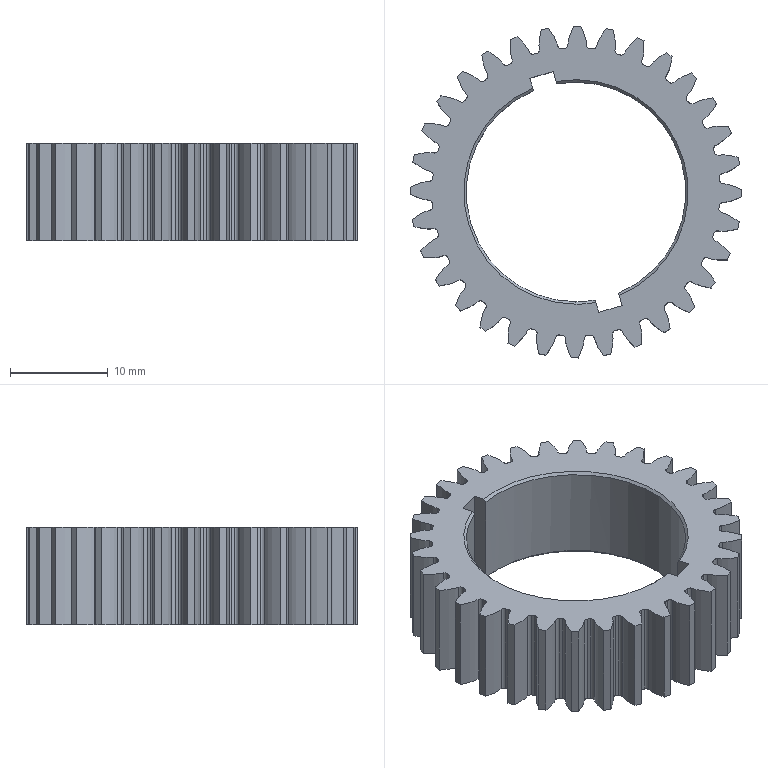Part | STEP file | GEAR_1_BODY-1 | 1 solid | 209 faces | box 34 x 34 x 10 mm | volume 3918 mm3 | spline 160 | cylinder 35 | plane 8 | cone 6 | commonest cylinder face diameters 29.5 x32 22.5 x3